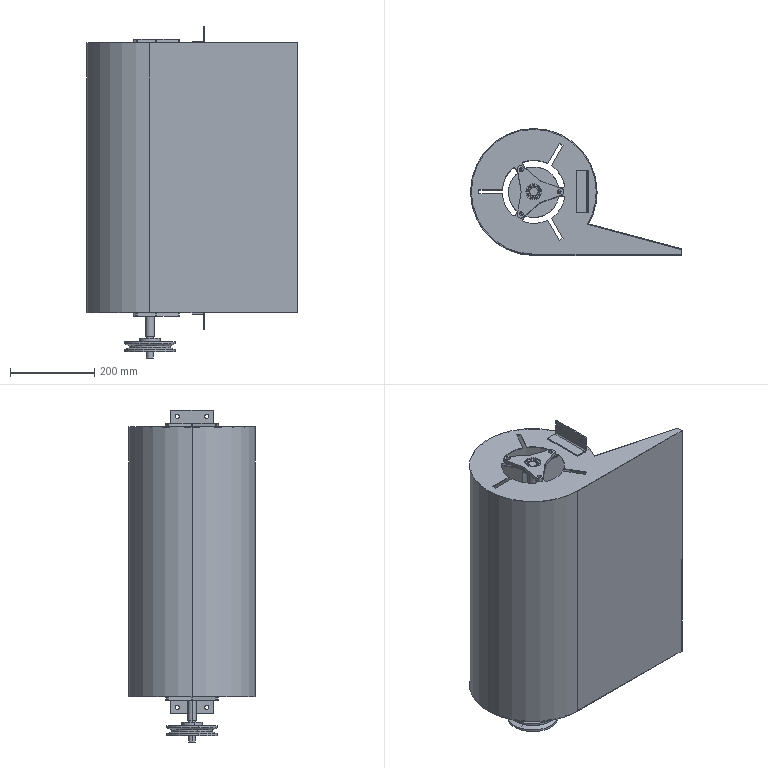Part | SolidWorks | 14 solids | 629 faces | box 500 x 300 x 787 mm | volume 3135900 mm3 | spline 220 | cylinder 205 | plane 192 | cone 12 | commonest cylinder face diameters 9 x32 20 x23 10 x16 37.8 x16 6 x14 130 x12